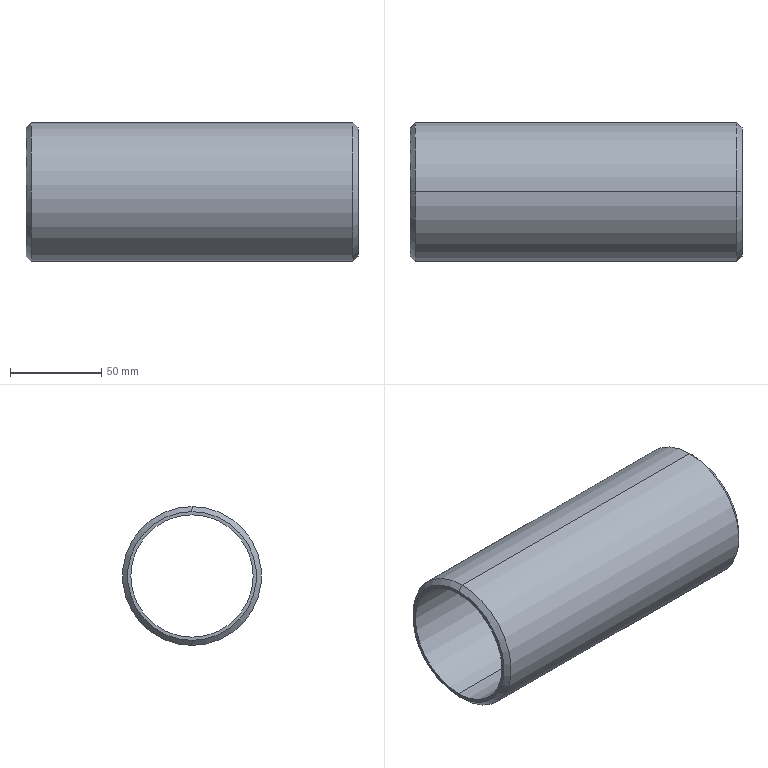Part | SolidWorks | features Chamfer 1, WeldMemberFeat 1, WeldmentFeature 1 | 1 solid | 10 faces | box 182 x 76.1 x 76.1 mm | volume 182460 mm3 | cone 4 | cylinder 4 | plane 2 | commonest cylinder face diameters 67.1 x2 76.1 x2
STEP:
#1=CARTESIAN_POINT('',(0.,0.,35.3));
#2=VERTEX_POINT('',#1);
#3=CARTESIAN_POINT('',(0.,0.,-35.3));
#4=VERTEX_POINT('',#3);
#5=CARTESIAN_POINT('',(0.,0.,0.));
#6=DIRECTION('',(-1.,0.,0.));
#7=DIRECTION('',(0.,0.,-1.));
#8=AXIS2_PLACEMENT_3D('',#5,#6,#7);
#9=CIRCLE('',#8,35.3);
#10=EDGE_CURVE('',#2,#4,#9,.T.);
#11=ORIENTED_EDGE('',*,*,#10,.F.);
#12=CARTESIAN_POINT('',(2.75,0.,38.05));
#13=VERTEX_POINT('',#12);
#14=CARTESIAN_POINT('',(2.75,0.,38.05));
#15=DIRECTION('',(0.7071,0.,0.7071));
#16=VECTOR('',#15,1000.);
#17=LINE('',#14,#16);
#18=EDGE_CURVE('',#2,#13,#17,.T.);
#19=ORIENTED_EDGE('',*,*,#18,.T.);
#20=CARTESIAN_POINT('',(2.75,0.,-38.05));
#21=VERTEX_POINT('',#20);
#22=CARTESIAN_POINT('',(2.75,0.,0.));
#23=DIRECTION('',(1.,0.,0.));
#24=DIRECTION('',(0.,0.,-1.));
#25=AXIS2_PLACEMENT_3D('',#22,#23,#24);
#26=CIRCLE('',#25,38.05);
#27=EDGE_CURVE('',#21,#13,#26,.T.);
#28=ORIENTED_EDGE('',*,*,#27,.F.);
#29=CARTESIAN_POINT('',(2.75,0.,-38.05));
#30=DIRECTION('',(0.7071,0.,-0.7071));
#31=VECTOR('',#30,1000.);
#32=LINE('',#29,#31);
#33=EDGE_CURVE('',#4,#21,#32,.T.);
#34=ORIENTED_EDGE('',*,*,#33,.F.);
#35=EDGE_LOOP('',(#11,#19,#28,#34));
#36=FACE_OUTER_BOUND('',#35,.T.);
#37=CARTESIAN_POINT('',(2.75,0.,0.));
#38=DIRECTION('',(1.,0.,0.));
#39=DIRECTION('',(0.,0.,-1.));
#40=AXIS2_PLACEMENT_3D('',#37,#38,#39);
#41=CONICAL_SURFACE('',#40,38.05,0.7854);
#42=ADVANCED_FACE('',(#36),#41,.T.);
#43=CARTESIAN_POINT('',(182.,0.,-35.3));
#44=VERTEX_POINT('',#43);
#45=CARTESIAN_POINT('',(182.,0.,35.3));
#46=VERTEX_POINT('',#45);
#47=CARTESIAN_POINT('',(182.,0.,0.));
#48=DIRECTION('',(1.,0.,0.));
#49=DIRECTION('',(0.,0.,-1.));
#50=AXIS2_PLACEMENT_3D('',#47,#48,#49);
#51=CIRCLE('',#50,35.3);
#52=EDGE_CURVE('',#44,#46,#51,.T.);
#53=ORIENTED_EDGE('',*,*,#52,.F.);
#54=CARTESIAN_POINT('',(179.25,0.,-38.05));
#55=VERTEX_POINT('',#54);
#56=CARTESIAN_POINT('',(182.,0.,-35.3));
#57=DIRECTION('',(-0.7071,0.,-0.7071));
#58=VECTOR('',#57,1000.);
#59=LINE('',#56,#58);
#60=EDGE_CURVE('',#44,#55,#59,.T.);
#61=ORIENTED_EDGE('',*,*,#60,.T.);
#62=CARTESIAN_POINT('',(179.25,0.,38.05));
#63=VERTEX_POINT('',#62);
#64=CARTESIAN_POINT('',(179.25,0.,0.));
#65=DIRECTION('',(-1.,0.,0.));
#66=DIRECTION('',(0.,0.,-1.));
#67=AXIS2_PLACEMENT_3D('',#64,#65,#66);
#68=CIRCLE('',#67,38.05);
#69=EDGE_CURVE('',#63,#55,#68,.T.);
#70=ORIENTED_EDGE('',*,*,#69,.F.);
#71=CARTESIAN_POINT('',(182.,0.,35.3));
#72=DIRECTION('',(-0.7071,0.,0.7071));
#73=VECTOR('',#72,1000.);
#74=LINE('',#71,#73);
#75=EDGE_CURVE('',#46,#63,#74,.T.);
#76=ORIENTED_EDGE('',*,*,#75,.F.);
#77=EDGE_LOOP('',(#53,#61,#70,#76));
#78=FACE_OUTER_BOUND('',#77,.T.);
#79=CARTESIAN_POINT('',(182.,0.,0.));
#80=DIRECTION('',(-1.,0.,0.));
#81=DIRECTION('',(0.,0.,1.));
#82=AXIS2_PLACEMENT_3D('',#79,#80,#81);
#83=CONICAL_SURFACE('',#82,35.3,0.7854);
#84=ADVANCED_FACE('',(#78),#83,.T.);
#85=ORIENTED_EDGE('',*,*,#69,.T.);
#86=CARTESIAN_POINT('',(182.,0.,-38.05));
#87=DIRECTION('',(-1.,0.,0.));
#88=VECTOR('',#87,1000.);
#89=LINE('',#86,#88);
#90=EDGE_CURVE('',#55,#21,#89,.T.);
#91=ORIENTED_EDGE('',*,*,#90,.T.);
#92=ORIENTED_EDGE('',*,*,#27,.T.);
#93=CARTESIAN_POINT('',(182.,0.,38.05));
#94=DIRECTION('',(-1.,0.,0.));
#95=VECTOR('',#94,1000.);
#96=LINE('',#93,#95);
#97=EDGE_CURVE('',#63,#13,#96,.T.);
#98=ORIENTED_EDGE('',*,*,#97,.F.);
#99=EDGE_LOOP('',(#85,#91,#92,#98));
#100=FACE_OUTER_BOUND('',#99,.T.);
#101=CARTESIAN_POINT('',(182.,0.,0.));
#102=DIRECTION('',(-1.,0.,0.));
#103=DIRECTION('',(0.,0.,1.));
#104=AXIS2_PLACEMENT_3D('',#101,#102,#103);
#105=CYLINDRICAL_SURFACE('',#104,38.05);
#106=ADVANCED_FACE('',(#100),#105,.T.);
#107=CARTESIAN_POINT('',(182.,0.,33.55));
#108=VERTEX_POINT('',#107);
#109=CARTESIAN_POINT('',(182.,0.,-33.55));
#110=VERTEX_POINT('',#109);
#111=CARTESIAN_POINT('',(182.,0.,0.));
#112=DIRECTION('',(1.,0.,0.));
#113=DIRECTION('',(0.,0.,-1.));
#114=AXIS2_PLACEMENT_3D('',#111,#112,#113);
#115=CIRCLE('',#114,33.55);
#116=EDGE_CURVE('',#108,#110,#115,.T.);
#117=ORIENTED_EDGE('',*,*,#116,.T.);
#118=CARTESIAN_POINT('',(0.,0.,-33.55));
#119=VERTEX_POINT('',#118);
#120=CARTESIAN_POINT('',(182.,0.,-33.55));
#121=DIRECTION('',(-1.,0.,0.));
#122=VECTOR('',#121,1000.);
#123=LINE('',#120,#122);
#124=EDGE_CURVE('',#110,#119,#123,.T.);
#125=ORIENTED_EDGE('',*,*,#124,.T.);
#126=CARTESIAN_POINT('',(0.,0.,33.55));
#127=VERTEX_POINT('',#126);
#128=CARTESIAN_POINT('',(0.,0.,0.));
#129=DIRECTION('',(1.,0.,0.));
#130=DIRECTION('',(0.,0.,-1.));
#131=AXIS2_PLACEMENT_3D('',#128,#129,#130);
#132=CIRCLE('',#131,33.55);
#133=EDGE_CURVE('',#127,#119,#132,.T.);
#134=ORIENTED_EDGE('',*,*,#133,.F.);
#135=CARTESIAN_POINT('',(182.,0.,33.55));
#136=DIRECTION('',(-1.,0.,0.));
#137=VECTOR('',#136,1000.);
#138=LINE('',#135,#137);
#139=EDGE_CURVE('',#108,#127,#138,.T.);
#140=ORIENTED_EDGE('',*,*,#139,.F.);
#141=EDGE_LOOP('',(#117,#125,#134,#140));
#142=FACE_OUTER_BOUND('',#141,.T.);
#143=CARTESIAN_POINT('',(182.,0.,0.));
#144=DIRECTION('',(-1.,0.,0.));
#145=DIRECTION('',(0.,0.,1.));
#146=AXIS2_PLACEMENT_3D('',#143,#144,#145);
#147=CYLINDRICAL_SURFACE('',#146,33.55);
#148=ADVANCED_FACE('',(#142),#147,.F.);
#149=ORIENTED_EDGE('',*,*,#124,.F.);
#150=CARTESIAN_POINT('',(182.,0.,0.));
#151=DIRECTION('',(1.,0.,0.));
#152=DIRECTION('',(0.,0.,-1.));
#153=AXIS2_PLACEMENT_3D('',#150,#151,#152);
#154=CIRCLE('',#153,33.55);
#155=EDGE_CURVE('',#110,#108,#154,.T.);
#156=ORIENTED_EDGE('',*,*,#155,.T.);
#157=ORIENTED_EDGE('',*,*,#139,.T.);
#158=CARTESIAN_POINT('',(0.,0.,0.));
#159=DIRECTION('',(1.,0.,0.));
#160=DIRECTION('',(0.,0.,-1.));
#161=AXIS2_PLACEMENT_3D('',#158,#159,#160);
#162=CIRCLE('',#161,33.55);
#163=EDGE_CURVE('',#119,#127,#162,.T.);
#164=ORIENTED_EDGE('',*,*,#163,.F.);
#165=EDGE_LOOP('',(#149,#156,#157,#164));
#166=FACE_OUTER_BOUND('',#165,.T.);
#167=CARTESIAN_POINT('',(182.,0.,0.));
#168=DIRECTION('',(-1.,0.,0.));
#169=DIRECTION('',(0.,0.,1.));
#170=AXIS2_PLACEMENT_3D('',#167,#168,#169);
#171=CYLINDRICAL_SURFACE('',#170,33.55);
#172=ADVANCED_FACE('',(#166),#171,.F.);
#173=ORIENTED_EDGE('',*,*,#90,.F.);
#174=CARTESIAN_POINT('',(179.25,0.,0.));
#175=DIRECTION('',(-1.,0.,0.));
#176=DIRECTION('',(0.,0.,-1.));
#177=AXIS2_PLACEMENT_3D('',#174,#175,#176);
#178=CIRCLE('',#177,38.05);
#179=EDGE_CURVE('',#55,#63,#178,.T.);
#180=ORIENTED_EDGE('',*,*,#179,.T.);
#181=ORIENTED_EDGE('',*,*,#97,.T.);
#182=CARTESIAN_POINT('',(2.75,0.,0.));
#183=DIRECTION('',(1.,0.,0.));
#184=DIRECTION('',(0.,0.,-1.));
#185=AXIS2_PLACEMENT_3D('',#182,#183,#184);
#186=CIRCLE('',#185,38.05);
#187=EDGE_CURVE('',#13,#21,#186,.T.);
#188=ORIENTED_EDGE('',*,*,#187,.T.);
#189=EDGE_LOOP('',(#173,#180,#181,#188));
#190=FACE_OUTER_BOUND('',#189,.T.);
#191=CARTESIAN_POINT('',(182.,0.,0.));
#192=DIRECTION('',(-1.,0.,0.));
#193=DIRECTION('',(0.,0.,1.));
#194=AXIS2_PLACEMENT_3D('',#191,#192,#193);
#195=CYLINDRICAL_SURFACE('',#194,38.05);
#196=ADVANCED_FACE('',(#190),#195,.T.);
#197=CARTESIAN_POINT('',(182.,0.,0.));
#198=DIRECTION('',(1.,0.,0.));
#199=DIRECTION('',(0.,0.,-1.));
#200=AXIS2_PLACEMENT_3D('',#197,#198,#199);
#201=CIRCLE('',#200,35.3);
#202=EDGE_CURVE('',#46,#44,#201,.T.);
#203=ORIENTED_EDGE('',*,*,#202,.T.);
#204=ORIENTED_EDGE('',*,*,#52,.T.);
#205=EDGE_LOOP('',(#203,#204));
#206=FACE_OUTER_BOUND('',#205,.T.);
#207=ORIENTED_EDGE('',*,*,#116,.F.);
#208=ORIENTED_EDGE('',*,*,#155,.F.);
#209=EDGE_LOOP('',(#207,#208));
#210=FACE_BOUND('',#209,.T.);
#211=CARTESIAN_POINT('',(182.,0.,0.));
#212=DIRECTION('',(1.,0.,0.));
#213=DIRECTION('',(0.,0.,-1.));
#214=AXIS2_PLACEMENT_3D('',#211,#212,#213);
#215=PLANE('',#214);
#216=ADVANCED_FACE('',(#206,#210),#215,.T.);
#217=CARTESIAN_POINT('',(0.,0.,0.));
#218=DIRECTION('',(-1.,0.,0.));
#219=DIRECTION('',(0.,0.,-1.));
#220=AXIS2_PLACEMENT_3D('',#217,#218,#219);
#221=CIRCLE('',#220,35.3);
#222=EDGE_CURVE('',#4,#2,#221,.T.);
#223=ORIENTED_EDGE('',*,*,#222,.T.);
#224=ORIENTED_EDGE('',*,*,#10,.T.);
#225=EDGE_LOOP('',(#223,#224));
#226=FACE_OUTER_BOUND('',#225,.T.);
#227=ORIENTED_EDGE('',*,*,#133,.T.);
#228=ORIENTED_EDGE('',*,*,#163,.T.);
#229=EDGE_LOOP('',(#227,#228));
#230=FACE_BOUND('',#229,.T.);
#231=CARTESIAN_POINT('',(0.,0.,0.));
#232=DIRECTION('',(1.,0.,0.));
#233=DIRECTION('',(0.,0.,-1.));
#234=AXIS2_PLACEMENT_3D('',#231,#232,#233);
#235=PLANE('',#234);
#236=ADVANCED_FACE('',(#226,#230),#235,.F.);
#237=ORIENTED_EDGE('',*,*,#60,.F.);
#238=ORIENTED_EDGE('',*,*,#202,.F.);
#239=ORIENTED_EDGE('',*,*,#75,.T.);
#240=ORIENTED_EDGE('',*,*,#179,.F.);
#241=EDGE_LOOP('',(#237,#238,#239,#240));
#242=FACE_OUTER_BOUND('',#241,.T.);
#243=CARTESIAN_POINT('',(182.,0.,0.));
#244=DIRECTION('',(-1.,0.,0.));
#245=DIRECTION('',(0.,0.,1.));
#246=AXIS2_PLACEMENT_3D('',#243,#244,#245);
#247=CONICAL_SURFACE('',#246,35.3,0.7854);
#248=ADVANCED_FACE('',(#242),#247,.T.);
#249=ORIENTED_EDGE('',*,*,#18,.F.);
#250=ORIENTED_EDGE('',*,*,#222,.F.);
#251=ORIENTED_EDGE('',*,*,#33,.T.);
#252=ORIENTED_EDGE('',*,*,#187,.F.);
#253=EDGE_LOOP('',(#249,#250,#251,#252));
#254=FACE_OUTER_BOUND('',#253,.T.);
#255=CARTESIAN_POINT('',(2.75,0.,0.));
#256=DIRECTION('',(1.,0.,0.));
#257=DIRECTION('',(0.,0.,-1.));
#258=AXIS2_PLACEMENT_3D('',#255,#256,#257);
#259=CONICAL_SURFACE('',#258,38.05,0.7854);
#260=ADVANCED_FACE('',(#254),#259,.T.);
#261=CLOSED_SHELL('',(#42,#84,#106,#148,#172,#196,#216,#236,#248,#260));
#262=MANIFOLD_SOLID_BREP('',#261);
#263=CARTESIAN_POINT('',(0.,0.,0.));
#264=DIRECTION('',(0.,0.,1.));
#265=DIRECTION('',(1.,0.,0.));
#266=AXIS2_PLACEMENT_3D('',#263,#264,#265);
#267=(LENGTH_UNIT()NAMED_UNIT(*)SI_UNIT(.MILLI.,.METRE.));
#268=UNCERTAINTY_MEASURE_WITH_UNIT(LENGTH_MEASURE(0.00001),#267,'','');
#269=(NAMED_UNIT(*)PLANE_ANGLE_UNIT()SI_UNIT($,.RADIAN.));
#270=(NAMED_UNIT(*)SI_UNIT($,.STERADIAN.)SOLID_ANGLE_UNIT());
#271=(GEOMETRIC_REPRESENTATION_CONTEXT(3)GLOBAL_UNCERTAINTY_ASSIGNED_CONTEXT((#268))GLOBAL_UNIT_ASSIGNED_CONTEXT((#267,#269,#270))REPRESENTATION_CONTEXT('',''));
#272=ADVANCED_BREP_SHAPE_REPRESENTATION('',(#262,#266),#271);